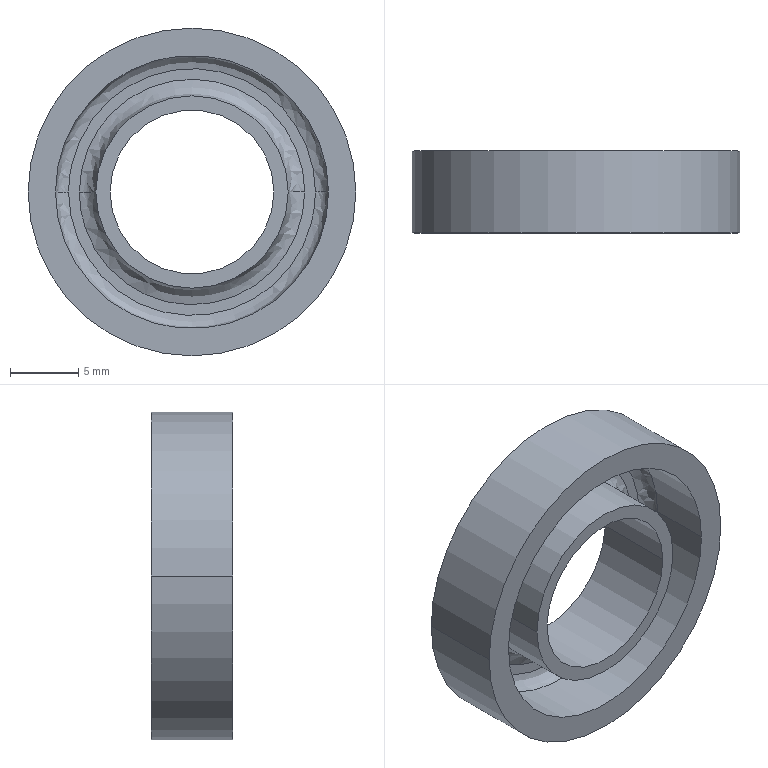Part | SolidWorks | features BaseBody 1 | 1 solid | 16 faces | box 24 x 6 x 24 mm | volume 1192 mm3 | cylinder 8 | spline 4 | plane 4 | commonest cylinder face diameters 12 x2 14.088 x2 20 x2 24 x2
STEP:
#1=CARTESIAN_POINT('',(-9.038,-85.,0.));
#2=VERTEX_POINT('',#1);
#3=CARTESIAN_POINT('',(9.038,-85.,0.));
#4=VERTEX_POINT('',#3);
#5=CARTESIAN_POINT('',(-9.038,-85.,0.));
#6=CARTESIAN_POINT('',(-9.038,-85.,-0.2762));
#7=CARTESIAN_POINT('',(-9.019,-85.,-0.6889));
#8=CARTESIAN_POINT('',(-8.964,-85.,-1.168));
#9=CARTESIAN_POINT('',(-8.928,-85.,-1.406));
#10=CARTESIAN_POINT('',(-8.911,-85.,-1.508));
#11=CARTESIAN_POINT('',(-8.899,-85.,-1.577));
#12=CARTESIAN_POINT('',(-8.893,-85.,-1.609));
#13=CARTESIAN_POINT('',(-8.834,-85.,-1.933));
#14=CARTESIAN_POINT('',(-8.733,-85.,-2.359));
#15=CARTESIAN_POINT('',(-8.58,-85.,-2.846));
#16=CARTESIAN_POINT('',(-8.495,-85.,-3.087));
#17=CARTESIAN_POINT('',(-8.456,-85.,-3.19));
#18=CARTESIAN_POINT('',(-8.43,-85.,-3.259));
#19=CARTESIAN_POINT('',(-8.417,-85.,-3.291));
#20=CARTESIAN_POINT('',(-8.291,-85.,-3.611));
#21=CARTESIAN_POINT('',(-8.102,-85.,-4.026));
#22=CARTESIAN_POINT('',(-7.845,-85.,-4.492));
#23=CARTESIAN_POINT('',(-7.727,-85.,-4.688));
#24=CARTESIAN_POINT('',(-7.647,-85.,-4.817));
#25=CARTESIAN_POINT('',(-7.607,-85.,-4.88));
#26=CARTESIAN_POINT('',(-7.223,-85.,-5.467));
#27=CARTESIAN_POINT('',(-6.832,-85.,-5.95));
#28=CARTESIAN_POINT('',(-6.17,-85.,-6.611));
#29=CARTESIAN_POINT('',(-5.824,-85.,-6.923));
#30=CARTESIAN_POINT('',(-5.394,-85.,-7.255));
#31=CARTESIAN_POINT('',(-5.204,-85.,-7.39));
#32=CARTESIAN_POINT('',(-5.076,-85.,-7.478));
#33=CARTESIAN_POINT('',(-5.009,-85.,-7.523));
#34=CARTESIAN_POINT('',(-4.69,-85.,-7.732));
#35=CARTESIAN_POINT('',(-4.296,-85.,-7.962));
#36=CARTESIAN_POINT('',(-3.818,-85.,-8.194));
#37=CARTESIAN_POINT('',(-3.574,-85.,-8.302));
#38=CARTESIAN_POINT('',(-3.468,-85.,-8.346));
#39=CARTESIAN_POINT('',(-3.398,-85.,-8.375));
#40=CARTESIAN_POINT('',(-3.361,-85.,-8.39));
#41=CARTESIAN_POINT('',(-3.054,-85.,-8.511));
#42=CARTESIAN_POINT('',(-2.64,-85.,-8.652));
#43=CARTESIAN_POINT('',(-2.146,-85.,-8.781));
#44=CARTESIAN_POINT('',(-1.896,-85.,-8.837));
#45=CARTESIAN_POINT('',(-1.788,-85.,-8.859));
#46=CARTESIAN_POINT('',(-1.717,-85.,-8.873));
#47=CARTESIAN_POINT('',(-1.678,-85.,-8.881));
#48=CARTESIAN_POINT('',(-1.101,-85.,-8.987));
#49=CARTESIAN_POINT('',(-0.5524,-85.,-9.038));
#50=CARTESIAN_POINT('',(0.2762,-85.,-9.038));
#51=CARTESIAN_POINT('',(0.6889,-85.,-9.019));
#52=CARTESIAN_POINT('',(1.168,-85.,-8.964));
#53=CARTESIAN_POINT('',(1.406,-85.,-8.928));
#54=CARTESIAN_POINT('',(1.508,-85.,-8.911));
#55=CARTESIAN_POINT('',(1.577,-85.,-8.899));
#56=CARTESIAN_POINT('',(1.609,-85.,-8.893));
#57=CARTESIAN_POINT('',(1.933,-85.,-8.834));
#58=CARTESIAN_POINT('',(2.359,-85.,-8.733));
#59=CARTESIAN_POINT('',(2.846,-85.,-8.58));
#60=CARTESIAN_POINT('',(3.087,-85.,-8.495));
#61=CARTESIAN_POINT('',(3.19,-85.,-8.456));
#62=CARTESIAN_POINT('',(3.259,-85.,-8.43));
#63=CARTESIAN_POINT('',(3.291,-85.,-8.417));
#64=CARTESIAN_POINT('',(3.611,-85.,-8.291));
#65=CARTESIAN_POINT('',(4.026,-85.,-8.102));
#66=CARTESIAN_POINT('',(4.492,-85.,-7.845));
#67=CARTESIAN_POINT('',(4.688,-85.,-7.727));
#68=CARTESIAN_POINT('',(4.817,-85.,-7.647));
#69=CARTESIAN_POINT('',(4.88,-85.,-7.607));
#70=CARTESIAN_POINT('',(5.467,-85.,-7.223));
#71=CARTESIAN_POINT('',(5.95,-85.,-6.832));
#72=CARTESIAN_POINT('',(6.611,-85.,-6.17));
#73=CARTESIAN_POINT('',(6.923,-85.,-5.824));
#74=CARTESIAN_POINT('',(7.255,-85.,-5.394));
#75=CARTESIAN_POINT('',(7.39,-85.,-5.204));
#76=CARTESIAN_POINT('',(7.478,-85.,-5.076));
#77=CARTESIAN_POINT('',(7.523,-85.,-5.009));
#78=CARTESIAN_POINT('',(7.732,-85.,-4.69));
#79=CARTESIAN_POINT('',(7.962,-85.,-4.296));
#80=CARTESIAN_POINT('',(8.194,-85.,-3.818));
#81=CARTESIAN_POINT('',(8.302,-85.,-3.574));
#82=CARTESIAN_POINT('',(8.346,-85.,-3.468));
#83=CARTESIAN_POINT('',(8.375,-85.,-3.398));
#84=CARTESIAN_POINT('',(8.39,-85.,-3.361));
#85=CARTESIAN_POINT('',(8.511,-85.,-3.054));
#86=CARTESIAN_POINT('',(8.652,-85.,-2.64));
#87=CARTESIAN_POINT('',(8.781,-85.,-2.146));
#88=CARTESIAN_POINT('',(8.837,-85.,-1.896));
#89=CARTESIAN_POINT('',(8.859,-85.,-1.788));
#90=CARTESIAN_POINT('',(8.873,-85.,-1.717));
#91=CARTESIAN_POINT('',(8.881,-85.,-1.678));
#92=CARTESIAN_POINT('',(8.987,-85.,-1.101));
#93=CARTESIAN_POINT('',(9.038,-85.,-0.5524));
#94=CARTESIAN_POINT('',(9.038,-85.,0.));
#95=B_SPLINE_CURVE_WITH_KNOTS('',3,(#5,#6,#7,#8,#9,#10,#11,#12,#13,#14,#15,#16,#17,#18,#19,#20,#21,#22,#23,#24,#25,#26,#27,#28,#29,#30,#31,#32,#33,#34,#35,#36,#37,#38,#39,#40,#41,#42,#43,#44,#45,#46,#47,#48,#49,#50,#51,#52,#53,#54,#55,#56,#57,#58,#59,#60,#61,#62,#63,#64,#65,#66,#67,#68,#69,#70,#71,#72,#73,#74,#75,#76,#77,#78,#79,#80,#81,#82,#83,#84,#85,#86,#87,#88,#89,#90,#91,#92,#93,#94),.UNSPECIFIED.,.F.,.F.,(4,1,1,1,2,2,1,1,1,2,2,1,1,2,2,2,1,1,2,2,1,1,1,2,2,1,1,1,2,2,2,1,1,1,2,2,1,1,1,2,2,1,1,2,2,2,1,1,2,2,1,1,1,2,2,1,1,1,2,2,4),(0.25,0.2656,0.2734,0.2773,0.2793,0.2813,0.2969,0.3047,0.3086,0.3105,0.3125,0.3281,0.3359,0.3398,0.3438,0.375,0.3906,0.3984,0.4023,0.4063,0.4219,0.4297,0.4336,0.4355,0.4375,0.4531,0.4609,0.4648,0.4668,0.4688,0.5,0.5156,0.5234,0.5273,0.5293,0.5313,0.5469,0.5547,0.5586,0.5605,0.5625,0.5781,0.5859,0.5898,0.5938,0.625,0.6406,0.6484,0.6523,0.6563,0.6719,0.6797,0.6836,0.6855,0.6875,0.7031,0.7109,0.7148,0.7168,0.7188,0.75),.UNSPECIFIED.);
#96=EDGE_CURVE('',#2,#4,#95,.T.);
#97=ORIENTED_EDGE('',*,*,#96,.F.);
#98=CARTESIAN_POINT('',(-10.,-85.962,0.));
#99=VERTEX_POINT('',#98);
#100=CARTESIAN_POINT('',(-9.038,-85.962,0.));
#101=DIRECTION('',(0.,0.,1.));
#102=DIRECTION('',(-1.,0.,0.));
#103=AXIS2_PLACEMENT_3D('',#100,#101,#102);
#104=CIRCLE('',#103,0.9623);
#105=EDGE_CURVE('',#2,#99,#104,.T.);
#106=ORIENTED_EDGE('',*,*,#105,.T.);
#107=CARTESIAN_POINT('',(10.,-85.962,0.));
#108=VERTEX_POINT('',#107);
#109=CARTESIAN_POINT('',(0.,-85.962,0.));
#110=DIRECTION('',(0.,-1.,0.));
#111=DIRECTION('',(-1.,0.,0.));
#112=AXIS2_PLACEMENT_3D('',#109,#110,#111);
#113=CIRCLE('',#112,10.);
#114=EDGE_CURVE('',#99,#108,#113,.T.);
#115=ORIENTED_EDGE('',*,*,#114,.T.);
#116=CARTESIAN_POINT('',(9.038,-85.962,0.));
#117=DIRECTION('',(0.,0.,-1.));
#118=DIRECTION('',(1.,0.,0.));
#119=AXIS2_PLACEMENT_3D('',#116,#117,#118);
#120=CIRCLE('',#119,0.9623);
#121=EDGE_CURVE('',#4,#108,#120,.T.);
#122=ORIENTED_EDGE('',*,*,#121,.F.);
#123=EDGE_LOOP('',(#97,#106,#115,#122));
#124=FACE_OUTER_BOUND('',#123,.T.);
#125=CARTESIAN_POINT('',(9.038,-85.,0.));
#126=CARTESIAN_POINT('',(9.038,-85.,-18.075));
#127=CARTESIAN_POINT('',(-9.038,-85.,-18.075));
#128=CARTESIAN_POINT('',(-9.038,-85.,0.));
#129=CARTESIAN_POINT('',(9.601,-85.,0.));
#130=CARTESIAN_POINT('',(9.601,-85.,-19.203));
#131=CARTESIAN_POINT('',(-9.601,-85.,-19.203));
#132=CARTESIAN_POINT('',(-9.601,-85.,0.));
#133=CARTESIAN_POINT('',(10.,-85.399,0.));
#134=CARTESIAN_POINT('',(10.,-85.399,-20.));
#135=CARTESIAN_POINT('',(-10.,-85.399,-20.));
#136=CARTESIAN_POINT('',(-10.,-85.399,0.));
#137=CARTESIAN_POINT('',(10.,-85.962,0.));
#138=CARTESIAN_POINT('',(10.,-85.962,-20.));
#139=CARTESIAN_POINT('',(-10.,-85.962,-20.));
#140=CARTESIAN_POINT('',(-10.,-85.962,0.));
#141=(BOUNDED_SURFACE()B_SPLINE_SURFACE(3,3,((#125,#126,#127,#128),(#129,#130,#131,#132),(#133,#134,#135,#136),(#137,#138,#139,#140)),.UNSPECIFIED.,.F.,.F.,.T.)B_SPLINE_SURFACE_WITH_KNOTS((4,4),(4,4),(0.,1.),(0.,1.),.UNSPECIFIED.)GEOMETRIC_REPRESENTATION_ITEM()RATIONAL_B_SPLINE_SURFACE(((1.,0.3333,0.3333,1.),(0.8047,0.2682,0.2682,0.8047),(0.8047,0.2682,0.2682,0.8047),(1.,0.3333,0.3333,1.)))REPRESENTATION_ITEM('')SURFACE());
#142=ADVANCED_FACE('',(#124),#141,.F.);
#143=CARTESIAN_POINT('',(-7.044,-86.21,0.));
#144=VERTEX_POINT('',#143);
#145=CARTESIAN_POINT('',(7.044,-86.21,0.));
#146=VERTEX_POINT('',#145);
#147=CARTESIAN_POINT('',(0.,-86.21,0.));
#148=DIRECTION('',(0.,-1.,0.));
#149=DIRECTION('',(-1.,0.,0.));
#150=AXIS2_PLACEMENT_3D('',#147,#148,#149);
#151=CIRCLE('',#150,7.044);
#152=EDGE_CURVE('',#144,#146,#151,.T.);
#153=ORIENTED_EDGE('',*,*,#152,.F.);
#154=CARTESIAN_POINT('',(-8.255,-85.,0.));
#155=VERTEX_POINT('',#154);
#156=CARTESIAN_POINT('',(-8.255,-86.21,0.));
#157=DIRECTION('',(0.,0.,1.));
#158=DIRECTION('',(-1.,0.,0.));
#159=AXIS2_PLACEMENT_3D('',#156,#157,#158);
#160=CIRCLE('',#159,1.21);
#161=EDGE_CURVE('',#144,#155,#160,.T.);
#162=ORIENTED_EDGE('',*,*,#161,.T.);
#163=CARTESIAN_POINT('',(8.255,-85.,0.));
#164=VERTEX_POINT('',#163);
#165=CARTESIAN_POINT('',(8.255,-85.,0.));
#166=CARTESIAN_POINT('',(8.255,-85.,-0.2523));
#167=CARTESIAN_POINT('',(8.237,-85.,-0.6292));
#168=CARTESIAN_POINT('',(8.187,-85.,-1.066));
#169=CARTESIAN_POINT('',(8.154,-85.,-1.284));
#170=CARTESIAN_POINT('',(8.139,-85.,-1.378));
#171=CARTESIAN_POINT('',(8.128,-85.,-1.44));
#172=CARTESIAN_POINT('',(8.123,-85.,-1.469));
#173=CARTESIAN_POINT('',(8.068,-85.,-1.765));
#174=CARTESIAN_POINT('',(7.976,-85.,-2.154));
#175=CARTESIAN_POINT('',(7.837,-85.,-2.599));
#176=CARTESIAN_POINT('',(7.758,-85.,-2.82));
#177=CARTESIAN_POINT('',(7.723,-85.,-2.914));
#178=CARTESIAN_POINT('',(7.699,-85.,-2.976));
#179=CARTESIAN_POINT('',(7.688,-85.,-3.006));
#180=CARTESIAN_POINT('',(7.572,-85.,-3.298));
#181=CARTESIAN_POINT('',(7.4,-85.,-3.677));
#182=CARTESIAN_POINT('',(7.165,-85.,-4.102));
#183=CARTESIAN_POINT('',(7.058,-85.,-4.281));
#184=CARTESIAN_POINT('',(6.985,-85.,-4.4));
#185=CARTESIAN_POINT('',(6.948,-85.,-4.457));
#186=CARTESIAN_POINT('',(6.597,-85.,-4.994));
#187=CARTESIAN_POINT('',(6.239,-85.,-5.434));
#188=CARTESIAN_POINT('',(5.635,-85.,-6.038));
#189=CARTESIAN_POINT('',(5.32,-85.,-6.323));
#190=CARTESIAN_POINT('',(4.926,-85.,-6.626));
#191=CARTESIAN_POINT('',(4.753,-85.,-6.749));
#192=CARTESIAN_POINT('',(4.636,-85.,-6.83));
#193=CARTESIAN_POINT('',(4.575,-85.,-6.871));
#194=CARTESIAN_POINT('',(4.284,-85.,-7.062));
#195=CARTESIAN_POINT('',(3.924,-85.,-7.272));
#196=CARTESIAN_POINT('',(3.487,-85.,-7.484));
#197=CARTESIAN_POINT('',(3.264,-85.,-7.582));
#198=CARTESIAN_POINT('',(3.168,-85.,-7.623));
#199=CARTESIAN_POINT('',(3.103,-85.,-7.649));
#200=CARTESIAN_POINT('',(3.07,-85.,-7.663));
#201=CARTESIAN_POINT('',(2.79,-85.,-7.773));
#202=CARTESIAN_POINT('',(2.411,-85.,-7.903));
#203=CARTESIAN_POINT('',(1.96,-85.,-8.02));
#204=CARTESIAN_POINT('',(1.732,-85.,-8.071));
#205=CARTESIAN_POINT('',(1.633,-85.,-8.091));
#206=CARTESIAN_POINT('',(1.568,-85.,-8.104));
#207=CARTESIAN_POINT('',(1.533,-85.,-8.111));
#208=CARTESIAN_POINT('',(1.006,-85.,-8.209));
#209=CARTESIAN_POINT('',(0.5045,-85.,-8.254));
#210=CARTESIAN_POINT('',(-0.2523,-85.,-8.255));
#211=CARTESIAN_POINT('',(-0.6292,-85.,-8.237));
#212=CARTESIAN_POINT('',(-1.066,-85.,-8.187));
#213=CARTESIAN_POINT('',(-1.284,-85.,-8.154));
#214=CARTESIAN_POINT('',(-1.378,-85.,-8.139));
#215=CARTESIAN_POINT('',(-1.44,-85.,-8.128));
#216=CARTESIAN_POINT('',(-1.469,-85.,-8.123));
#217=CARTESIAN_POINT('',(-1.765,-85.,-8.068));
#218=CARTESIAN_POINT('',(-2.154,-85.,-7.976));
#219=CARTESIAN_POINT('',(-2.599,-85.,-7.837));
#220=CARTESIAN_POINT('',(-2.82,-85.,-7.758));
#221=CARTESIAN_POINT('',(-2.914,-85.,-7.723));
#222=CARTESIAN_POINT('',(-2.976,-85.,-7.699));
#223=CARTESIAN_POINT('',(-3.006,-85.,-7.688));
#224=CARTESIAN_POINT('',(-3.298,-85.,-7.572));
#225=CARTESIAN_POINT('',(-3.677,-85.,-7.4));
#226=CARTESIAN_POINT('',(-4.102,-85.,-7.165));
#227=CARTESIAN_POINT('',(-4.281,-85.,-7.058));
#228=CARTESIAN_POINT('',(-4.4,-85.,-6.985));
#229=CARTESIAN_POINT('',(-4.457,-85.,-6.948));
#230=CARTESIAN_POINT('',(-4.994,-85.,-6.597));
#231=CARTESIAN_POINT('',(-5.434,-85.,-6.239));
#232=CARTESIAN_POINT('',(-6.038,-85.,-5.635));
#233=CARTESIAN_POINT('',(-6.323,-85.,-5.32));
#234=CARTESIAN_POINT('',(-6.626,-85.,-4.926));
#235=CARTESIAN_POINT('',(-6.749,-85.,-4.753));
#236=CARTESIAN_POINT('',(-6.83,-85.,-4.636));
#237=CARTESIAN_POINT('',(-6.871,-85.,-4.575));
#238=CARTESIAN_POINT('',(-7.062,-85.,-4.284));
#239=CARTESIAN_POINT('',(-7.272,-85.,-3.924));
#240=CARTESIAN_POINT('',(-7.484,-85.,-3.487));
#241=CARTESIAN_POINT('',(-7.582,-85.,-3.264));
#242=CARTESIAN_POINT('',(-7.623,-85.,-3.168));
#243=CARTESIAN_POINT('',(-7.649,-85.,-3.103));
#244=CARTESIAN_POINT('',(-7.663,-85.,-3.07));
#245=CARTESIAN_POINT('',(-7.773,-85.,-2.79));
#246=CARTESIAN_POINT('',(-7.903,-85.,-2.411));
#247=CARTESIAN_POINT('',(-8.02,-85.,-1.96));
#248=CARTESIAN_POINT('',(-8.071,-85.,-1.732));
#249=CARTESIAN_POINT('',(-8.091,-85.,-1.633));
#250=CARTESIAN_POINT('',(-8.104,-85.,-1.568));
#251=CARTESIAN_POINT('',(-8.111,-85.,-1.533));
#252=CARTESIAN_POINT('',(-8.209,-85.,-1.006));
#253=CARTESIAN_POINT('',(-8.254,-85.,-0.5045));
#254=CARTESIAN_POINT('',(-8.255,-85.,0.));
#255=B_SPLINE_CURVE_WITH_KNOTS('',3,(#165,#166,#167,#168,#169,#170,#171,#172,#173,#174,#175,#176,#177,#178,#179,#180,#181,#182,#183,#184,#185,#186,#187,#188,#189,#190,#191,#192,#193,#194,#195,#196,#197,#198,#199,#200,#201,#202,#203,#204,#205,#206,#207,#208,#209,#210,#211,#212,#213,#214,#215,#216,#217,#218,#219,#220,#221,#222,#223,#224,#225,#226,#227,#228,#229,#230,#231,#232,#233,#234,#235,#236,#237,#238,#239,#240,#241,#242,#243,#244,#245,#246,#247,#248,#249,#250,#251,#252,#253,#254),.UNSPECIFIED.,.F.,.F.,(4,1,1,1,2,2,1,1,1,2,2,1,1,2,2,2,1,1,2,2,1,1,1,2,2,1,1,1,2,2,2,1,1,1,2,2,1,1,1,2,2,1,1,2,2,2,1,1,2,2,1,1,1,2,2,1,1,1,2,2,4),(0.25,0.2656,0.2734,0.2773,0.2793,0.2812,0.2969,0.3047,0.3086,0.3105,0.3125,0.3281,0.3359,0.3398,0.3437,0.375,0.3906,0.3984,0.4023,0.4062,0.4219,0.4297,0.4336,0.4355,0.4375,0.4531,0.4609,0.4648,0.4668,0.4687,0.5,0.5156,0.5234,0.5273,0.5293,0.5313,0.5469,0.5547,0.5586,0.5605,0.5625,0.5781,0.5859,0.5898,0.5938,0.625,0.6406,0.6484,0.6523,0.6563,0.6719,0.6797,0.6836,0.6855,0.6875,0.7031,0.7109,0.7148,0.7168,0.7188,0.75),.UNSPECIFIED.);
#256=EDGE_CURVE('',#164,#155,#255,.T.);
#257=ORIENTED_EDGE('',*,*,#256,.F.);
#258=CARTESIAN_POINT('',(8.255,-86.21,0.));
#259=DIRECTION('',(0.,0.,-1.));
#260=DIRECTION('',(1.,0.,0.));
#261=AXIS2_PLACEMENT_3D('',#258,#259,#260);
#262=CIRCLE('',#261,1.21);
#263=EDGE_CURVE('',#146,#164,#262,.T.);
#264=ORIENTED_EDGE('',*,*,#263,.F.);
#265=EDGE_LOOP('',(#153,#162,#257,#264));
#266=FACE_OUTER_BOUND('',#265,.T.);
#267=CARTESIAN_POINT('',(7.044,-86.21,0.));
#268=CARTESIAN_POINT('',(7.044,-86.21,-14.088));
#269=CARTESIAN_POINT('',(-7.044,-86.21,-14.088));
#270=CARTESIAN_POINT('',(-7.044,-86.21,0.));
#271=CARTESIAN_POINT('',(7.044,-85.501,0.));
#272=CARTESIAN_POINT('',(7.044,-85.501,-14.088));
#273=CARTESIAN_POINT('',(-7.044,-85.501,-14.088));
#274=CARTESIAN_POINT('',(-7.044,-85.501,0.));
#275=CARTESIAN_POINT('',(7.546,-85.,0.));
#276=CARTESIAN_POINT('',(7.546,-85.,-15.091));
#277=CARTESIAN_POINT('',(-7.546,-85.,-15.091));
#278=CARTESIAN_POINT('',(-7.546,-85.,0.));
#279=CARTESIAN_POINT('',(8.255,-85.,0.));
#280=CARTESIAN_POINT('',(8.255,-85.,-16.509));
#281=CARTESIAN_POINT('',(-8.255,-85.,-16.509));
#282=CARTESIAN_POINT('',(-8.255,-85.,0.));
#283=(BOUNDED_SURFACE()B_SPLINE_SURFACE(3,3,((#267,#268,#269,#270),(#271,#272,#273,#274),(#275,#276,#277,#278),(#279,#280,#281,#282)),.UNSPECIFIED.,.F.,.F.,.F.)B_SPLINE_SURFACE_WITH_KNOTS((4,4),(4,4),(0.,1.),(0.,1.),.UNSPECIFIED.)GEOMETRIC_REPRESENTATION_ITEM()RATIONAL_B_SPLINE_SURFACE(((1.,0.3333,0.3333,1.),(0.8047,0.2682,0.2682,0.8047),(0.8047,0.2682,0.2682,0.8047),(1.,0.3333,0.3333,1.)))REPRESENTATION_ITEM('')SURFACE());
#284=ADVANCED_FACE('',(#266),#283,.F.);
#285=CARTESIAN_POINT('',(-12.,-90.5,0.));
#286=VERTEX_POINT('',#285);
#287=CARTESIAN_POINT('',(12.,-90.5,0.));
#288=VERTEX_POINT('',#287);
#289=CARTESIAN_POINT('',(0.,-90.5,0.));
#290=DIRECTION('',(0.,1.,0.));
#291=DIRECTION('',(-1.,0.,0.));
#292=AXIS2_PLACEMENT_3D('',#289,#290,#291);
#293=CIRCLE('',#292,12.);
#294=EDGE_CURVE('',#286,#288,#293,.T.);
#295=ORIENTED_EDGE('',*,*,#294,.T.);
#296=CARTESIAN_POINT('',(12.,-84.5,0.));
#297=VERTEX_POINT('',#296);
#298=CARTESIAN_POINT('',(12.,-83.5,0.));
#299=DIRECTION('',(0.,1.,0.));
#300=VECTOR('',#299,1000.);
#301=LINE('',#298,#300);
#302=EDGE_CURVE('',#288,#297,#301,.T.);
#303=ORIENTED_EDGE('',*,*,#302,.T.);
#304=CARTESIAN_POINT('',(-12.,-84.5,0.));
#305=VERTEX_POINT('',#304);
#306=CARTESIAN_POINT('',(0.,-84.5,0.));
#307=DIRECTION('',(0.,-1.,0.));
#308=DIRECTION('',(-1.,0.,0.));
#309=AXIS2_PLACEMENT_3D('',#306,#307,#308);
#310=CIRCLE('',#309,12.);
#311=EDGE_CURVE('',#297,#305,#310,.T.);
#312=ORIENTED_EDGE('',*,*,#311,.T.);
#313=CARTESIAN_POINT('',(-12.,-83.5,0.));
#314=DIRECTION('',(0.,1.,0.));
#315=VECTOR('',#314,1000.);
#316=LINE('',#313,#315);
#317=EDGE_CURVE('',#286,#305,#316,.T.);
#318=ORIENTED_EDGE('',*,*,#317,.F.);
#319=EDGE_LOOP('',(#295,#303,#312,#318));
#320=FACE_OUTER_BOUND('',#319,.T.);
#321=CARTESIAN_POINT('',(0.,-83.5,0.));
#322=DIRECTION('',(0.,1.,0.));
#323=DIRECTION('',(-1.,0.,0.));
#324=AXIS2_PLACEMENT_3D('',#321,#322,#323);
#325=CYLINDRICAL_SURFACE('',#324,12.);
#326=ADVANCED_FACE('',(#320),#325,.T.);
#327=CARTESIAN_POINT('',(6.,-90.5,0.));
#328=VERTEX_POINT('',#327);
#329=CARTESIAN_POINT('',(-6.,-90.5,0.));
#330=VERTEX_POINT('',#329);
#331=CARTESIAN_POINT('',(0.,-90.5,0.));
#332=DIRECTION('',(0.,1.,0.));
#333=DIRECTION('',(-1.,0.,0.));
#334=AXIS2_PLACEMENT_3D('',#331,#332,#333);
#335=CIRCLE('',#334,6.);
#336=EDGE_CURVE('',#328,#330,#335,.T.);
#337=ORIENTED_EDGE('',*,*,#336,.F.);
#338=CARTESIAN_POINT('',(6.,-84.5,0.));
#339=VERTEX_POINT('',#338);
#340=CARTESIAN_POINT('',(6.,-83.5,0.));
#341=DIRECTION('',(0.,1.,0.));
#342=VECTOR('',#341,1000.);
#343=LINE('',#340,#342);
#344=EDGE_CURVE('',#328,#339,#343,.T.);
#345=ORIENTED_EDGE('',*,*,#344,.T.);
#346=CARTESIAN_POINT('',(-6.,-84.5,0.));
#347=VERTEX_POINT('',#346);
#348=CARTESIAN_POINT('',(0.,-84.5,0.));
#349=DIRECTION('',(0.,-1.,0.));
#350=DIRECTION('',(-1.,0.,0.));
#351=AXIS2_PLACEMENT_3D('',#348,#349,#350);
#352=CIRCLE('',#351,6.);
#353=EDGE_CURVE('',#347,#339,#352,.T.);
#354=ORIENTED_EDGE('',*,*,#353,.F.);
#355=CARTESIAN_POINT('',(-6.,-83.5,0.));
#356=DIRECTION('',(0.,1.,0.));
#357=VECTOR('',#356,1000.);
#358=LINE('',#355,#357);
#359=EDGE_CURVE('',#330,#347,#358,.T.);
#360=ORIENTED_EDGE('',*,*,#359,.F.);
#361=EDGE_LOOP('',(#337,#345,#354,#360));
#362=FACE_OUTER_BOUND('',#361,.T.);
#363=CARTESIAN_POINT('',(0.,-83.5,0.));
#364=DIRECTION('',(0.,1.,0.));
#365=DIRECTION('',(-1.,0.,0.));
#366=AXIS2_PLACEMENT_3D('',#363,#364,#365);
#367=CYLINDRICAL_SURFACE('',#366,6.);
#368=ADVANCED_FACE('',(#362),#367,.F.);
#369=CARTESIAN_POINT('',(10.,-90.5,0.));
#370=VERTEX_POINT('',#369);
#371=CARTESIAN_POINT('',(-10.,-90.5,0.));
#372=VERTEX_POINT('',#371);
#373=CARTESIAN_POINT('',(0.,-90.5,0.));
#374=DIRECTION('',(0.,1.,0.));
#375=DIRECTION('',(-1.,0.,0.));
#376=AXIS2_PLACEMENT_3D('',#373,#374,#375);
#377=CIRCLE('',#376,10.);
#378=EDGE_CURVE('',#370,#372,#377,.T.);
#379=ORIENTED_EDGE('',*,*,#378,.F.);
#380=CARTESIAN_POINT('',(10.,-83.5,0.));
#381=DIRECTION('',(0.,1.,0.));
#382=VECTOR('',#381,1000.);
#383=LINE('',#380,#382);
#384=EDGE_CURVE('',#370,#108,#383,.T.);
#385=ORIENTED_EDGE('',*,*,#384,.T.);
#386=ORIENTED_EDGE('',*,*,#114,.F.);
#387=CARTESIAN_POINT('',(-10.,-83.5,0.));
#388=DIRECTION('',(0.,1.,0.));
#389=VECTOR('',#388,1000.);
#390=LINE('',#387,#389);
#391=EDGE_CURVE('',#372,#99,#390,.T.);
#392=ORIENTED_EDGE('',*,*,#391,.F.);
#393=EDGE_LOOP('',(#379,#385,#386,#392));
#394=FACE_OUTER_BOUND('',#393,.T.);
#395=CARTESIAN_POINT('',(0.,-83.5,0.));
#396=DIRECTION('',(0.,1.,0.));
#397=DIRECTION('',(-1.,0.,0.));
#398=AXIS2_PLACEMENT_3D('',#395,#396,#397);
#399=CYLINDRICAL_SURFACE('',#398,10.);
#400=ADVANCED_FACE('',(#394),#399,.F.);
#401=CARTESIAN_POINT('',(7.044,-90.5,0.));
#402=VERTEX_POINT('',#401);
#403=CARTESIAN_POINT('',(-7.044,-90.5,0.));
#404=VERTEX_POINT('',#403);
#405=CARTESIAN_POINT('',(0.,-90.5,0.));
#406=DIRECTION('',(0.,-1.,0.));
#407=DIRECTION('',(-1.,0.,0.));
#408=AXIS2_PLACEMENT_3D('',#405,#406,#407);
#409=CIRCLE('',#408,7.044);
#410=EDGE_CURVE('',#402,#404,#409,.T.);
#411=ORIENTED_EDGE('',*,*,#410,.F.);
#412=CARTESIAN_POINT('',(7.044,-83.5,0.));
#413=DIRECTION('',(0.,1.,0.));
#414=VECTOR('',#413,1000.);
#415=LINE('',#412,#414);
#416=EDGE_CURVE('',#402,#146,#415,.T.);
#417=ORIENTED_EDGE('',*,*,#416,.T.);
#418=CARTESIAN_POINT('',(0.,-86.21,0.));
#419=DIRECTION('',(0.,-1.,0.));
#420=DIRECTION('',(-1.,0.,0.));
#421=AXIS2_PLACEMENT_3D('',#418,#419,#420);
#422=CIRCLE('',#421,7.044);
#423=EDGE_CURVE('',#146,#144,#422,.T.);
#424=ORIENTED_EDGE('',*,*,#423,.T.);
#425=CARTESIAN_POINT('',(-7.044,-83.5,0.));
#426=DIRECTION('',(0.,1.,0.));
#427=VECTOR('',#426,1000.);
#428=LINE('',#425,#427);
#429=EDGE_CURVE('',#404,#144,#428,.T.);
#430=ORIENTED_EDGE('',*,*,#429,.F.);
#431=EDGE_LOOP('',(#411,#417,#424,#430));
#432=FACE_OUTER_BOUND('',#431,.T.);
#433=CARTESIAN_POINT('',(0.,-83.5,0.));
#434=DIRECTION('',(0.,1.,0.));
#435=DIRECTION('',(-1.,0.,0.));
#436=AXIS2_PLACEMENT_3D('',#433,#434,#435);
#437=CYLINDRICAL_SURFACE('',#436,7.044);
#438=ADVANCED_FACE('',(#432),#437,.T.);
#439=ORIENTED_EDGE('',*,*,#302,.F.);
#440=CARTESIAN_POINT('',(0.,-90.5,0.));
#441=DIRECTION('',(0.,1.,0.));
#442=DIRECTION('',(-1.,0.,0.));
#443=AXIS2_PLACEMENT_3D('',#440,#441,#442);
#444=CIRCLE('',#443,12.);
#445=EDGE_CURVE('',#288,#286,#444,.T.);
#446=ORIENTED_EDGE('',*,*,#445,.T.);
#447=ORIENTED_EDGE('',*,*,#317,.T.);
#448=CARTESIAN_POINT('',(0.,-84.5,0.));
#449=DIRECTION('',(0.,-1.,0.));
#450=DIRECTION('',(-1.,0.,0.));
#451=AXIS2_PLACEMENT_3D('',#448,#449,#450);
#452=CIRCLE('',#451,12.);
#453=EDGE_CURVE('',#305,#297,#452,.T.);
#454=ORIENTED_EDGE('',*,*,#453,.T.);
#455=EDGE_LOOP('',(#439,#446,#447,#454));
#456=FACE_OUTER_BOUND('',#455,.T.);
#457=CARTESIAN_POINT('',(0.,-83.5,0.));
#458=DIRECTION('',(0.,1.,0.));
#459=DIRECTION('',(-1.,0.,0.));
#460=AXIS2_PLACEMENT_3D('',#457,#458,#459);
#461=CYLINDRICAL_SURFACE('',#460,12.);
#462=ADVANCED_FACE('',(#456),#461,.T.);
#463=ORIENTED_EDGE('',*,*,#353,.T.);
#464=CARTESIAN_POINT('',(0.,-84.5,0.));
#465=DIRECTION('',(0.,-1.,0.));
#466=DIRECTION('',(-1.,0.,0.));
#467=AXIS2_PLACEMENT_3D('',#464,#465,#466);
#468=CIRCLE('',#467,6.);
#469=EDGE_CURVE('',#339,#347,#468,.T.);
#470=ORIENTED_EDGE('',*,*,#469,.T.);
#471=EDGE_LOOP('',(#463,#470));
#472=FACE_BOUND('',#471,.T.);
#473=ORIENTED_EDGE('',*,*,#453,.F.);
#474=ORIENTED_EDGE('',*,*,#311,.F.);
#475=EDGE_LOOP('',(#473,#474));
#476=FACE_OUTER_BOUND('',#475,.T.);
#477=CARTESIAN_POINT('',(0.,-84.5,6.));
#478=DIRECTION('',(0.,1.,0.));
#479=DIRECTION('',(-1.,0.,0.));
#480=AXIS2_PLACEMENT_3D('',#477,#478,#479);
#481=PLANE('',#480);
#482=ADVANCED_FACE('',(#472,#476),#481,.T.);
#483=ORIENTED_EDGE('',*,*,#294,.F.);
#484=ORIENTED_EDGE('',*,*,#445,.F.);
#485=EDGE_LOOP('',(#483,#484));
#486=FACE_OUTER_BOUND('',#485,.T.);
#487=CARTESIAN_POINT('',(0.,-90.5,0.));
#488=DIRECTION('',(0.,1.,0.));
#489=DIRECTION('',(-1.,0.,0.));
#490=AXIS2_PLACEMENT_3D('',#487,#488,#489);
#491=CIRCLE('',#490,10.);
#492=EDGE_CURVE('',#372,#370,#491,.T.);
#493=ORIENTED_EDGE('',*,*,#492,.T.);
#494=ORIENTED_EDGE('',*,*,#378,.T.);
#495=EDGE_LOOP('',(#493,#494));
#496=FACE_BOUND('',#495,.T.);
#497=CARTESIAN_POINT('',(0.,-90.5,12.));
#498=DIRECTION('',(0.,-1.,0.));
#499=DIRECTION('',(1.,0.,0.));
#500=AXIS2_PLACEMENT_3D('',#497,#498,#499);
#501=PLANE('',#500);
#502=ADVANCED_FACE('',(#486,#496),#501,.T.);
#503=ORIENTED_EDGE('',*,*,#344,.F.);
#504=CARTESIAN_POINT('',(0.,-90.5,0.));
#505=DIRECTION('',(0.,1.,0.));
#506=DIRECTION('',(-1.,0.,0.));
#507=AXIS2_PLACEMENT_3D('',#504,#505,#506);
#508=CIRCLE('',#507,6.);
#509=EDGE_CURVE('',#330,#328,#508,.T.);
#510=ORIENTED_EDGE('',*,*,#509,.F.);
#511=ORIENTED_EDGE('',*,*,#359,.T.);
#512=ORIENTED_EDGE('',*,*,#469,.F.);
#513=EDGE_LOOP('',(#503,#510,#511,#512));
#514=FACE_OUTER_BOUND('',#513,.T.);
#515=CARTESIAN_POINT('',(0.,-83.5,0.));
#516=DIRECTION('',(0.,1.,0.));
#517=DIRECTION('',(-1.,0.,0.));
#518=AXIS2_PLACEMENT_3D('',#515,#516,#517);
#519=CYLINDRICAL_SURFACE('',#518,6.);
#520=ADVANCED_FACE('',(#514),#519,.F.);
#521=ORIENTED_EDGE('',*,*,#384,.F.);
#522=ORIENTED_EDGE('',*,*,#492,.F.);
#523=ORIENTED_EDGE('',*,*,#391,.T.);
#524=CARTESIAN_POINT('',(0.,-85.962,0.));
#525=DIRECTION('',(0.,-1.,0.));
#526=DIRECTION('',(-1.,0.,0.));
#527=AXIS2_PLACEMENT_3D('',#524,#525,#526);
#528=CIRCLE('',#527,10.);
#529=EDGE_CURVE('',#108,#99,#528,.T.);
#530=ORIENTED_EDGE('',*,*,#529,.F.);
#531=EDGE_LOOP('',(#521,#522,#523,#530));
#532=FACE_OUTER_BOUND('',#531,.T.);
#533=CARTESIAN_POINT('',(0.,-83.5,0.));
#534=DIRECTION('',(0.,1.,0.));
#535=DIRECTION('',(-1.,0.,0.));
#536=AXIS2_PLACEMENT_3D('',#533,#534,#535);
#537=CYLINDRICAL_SURFACE('',#536,10.);
#538=ADVANCED_FACE('',(#532),#537,.F.);
#539=CARTESIAN_POINT('',(0.,-90.5,0.));
#540=DIRECTION('',(0.,-1.,0.));
#541=DIRECTION('',(-1.,0.,0.));
#542=AXIS2_PLACEMENT_3D('',#539,#540,#541);
#543=CIRCLE('',#542,7.044);
#544=EDGE_CURVE('',#404,#402,#543,.T.);
#545=ORIENTED_EDGE('',*,*,#544,.T.);
#546=ORIENTED_EDGE('',*,*,#410,.T.);
#547=EDGE_LOOP('',(#545,#546));
#548=FACE_OUTER_BOUND('',#547,.T.);
#549=ORIENTED_EDGE('',*,*,#509,.T.);
#550=ORIENTED_EDGE('',*,*,#336,.T.);
#551=EDGE_LOOP('',(#549,#550));
#552=FACE_BOUND('',#551,.T.);
#553=CARTESIAN_POINT('',(0.,-90.5,7.044));
#554=DIRECTION('',(0.,-1.,0.));
#555=DIRECTION('',(1.,0.,0.));
#556=AXIS2_PLACEMENT_3D('',#553,#554,#555);
#557=PLANE('',#556);
#558=ADVANCED_FACE('',(#548,#552),#557,.T.);
#559=ORIENTED_EDGE('',*,*,#105,.F.);
#560=CARTESIAN_POINT('',(9.038,-85.,0.));
#561=CARTESIAN_POINT('',(9.038,-85.,0.2762));
#562=CARTESIAN_POINT('',(9.019,-85.,0.6889));
#563=CARTESIAN_POINT('',(8.964,-85.,1.168));
#564=CARTESIAN_POINT('',(8.928,-85.,1.406));
#565=CARTESIAN_POINT('',(8.911,-85.,1.508));
#566=CARTESIAN_POINT('',(8.899,-85.,1.577));
#567=CARTESIAN_POINT('',(8.893,-85.,1.609));
#568=CARTESIAN_POINT('',(8.834,-85.,1.933));
#569=CARTESIAN_POINT('',(8.733,-85.,2.359));
#570=CARTESIAN_POINT('',(8.58,-85.,2.846));
#571=CARTESIAN_POINT('',(8.495,-85.,3.087));
#572=CARTESIAN_POINT('',(8.456,-85.,3.19));
#573=CARTESIAN_POINT('',(8.43,-85.,3.259));
#574=CARTESIAN_POINT('',(8.417,-85.,3.291));
#575=CARTESIAN_POINT('',(8.291,-85.,3.611));
#576=CARTESIAN_POINT('',(8.102,-85.,4.026));
#577=CARTESIAN_POINT('',(7.845,-85.,4.492));
#578=CARTESIAN_POINT('',(7.727,-85.,4.688));
#579=CARTESIAN_POINT('',(7.647,-85.,4.817));
#580=CARTESIAN_POINT('',(7.607,-85.,4.88));
#581=CARTESIAN_POINT('',(7.223,-85.,5.467));
#582=CARTESIAN_POINT('',(6.832,-85.,5.95));
#583=CARTESIAN_POINT('',(6.17,-85.,6.611));
#584=CARTESIAN_POINT('',(5.824,-85.,6.923));
#585=CARTESIAN_POINT('',(5.394,-85.,7.255));
#586=CARTESIAN_POINT('',(5.204,-85.,7.39));
#587=CARTESIAN_POINT('',(5.076,-85.,7.478));
#588=CARTESIAN_POINT('',(5.009,-85.,7.523));
#589=CARTESIAN_POINT('',(4.69,-85.,7.732));
#590=CARTESIAN_POINT('',(4.296,-85.,7.962));
#591=CARTESIAN_POINT('',(3.818,-85.,8.194));
#592=CARTESIAN_POINT('',(3.574,-85.,8.302));
#593=CARTESIAN_POINT('',(3.468,-85.,8.346));
#594=CARTESIAN_POINT('',(3.398,-85.,8.375));
#595=CARTESIAN_POINT('',(3.361,-85.,8.39));
#596=CARTESIAN_POINT('',(3.054,-85.,8.511));
#597=CARTESIAN_POINT('',(2.64,-85.,8.652));
#598=CARTESIAN_POINT('',(2.146,-85.,8.781));
#599=CARTESIAN_POINT('',(1.896,-85.,8.837));
#600=CARTESIAN_POINT('',(1.788,-85.,8.859));
#601=CARTESIAN_POINT('',(1.717,-85.,8.873));
#602=CARTESIAN_POINT('',(1.678,-85.,8.881));
#603=CARTESIAN_POINT('',(1.101,-85.,8.987));
#604=CARTESIAN_POINT('',(0.553,-85.,9.038));
#605=CARTESIAN_POINT('',(-0.2765,-85.,9.038));
#606=CARTESIAN_POINT('',(-0.5515,-85.,9.025));
#607=CARTESIAN_POINT('',(-0.9626,-85.,8.987));
#608=CARTESIAN_POINT('',(-1.168,-85.,8.964));
#609=CARTESIAN_POINT('',(-1.406,-85.,8.928));
#610=CARTESIAN_POINT('',(-1.509,-85.,8.911));
#611=CARTESIAN_POINT('',(-1.577,-85.,8.899));
#612=CARTESIAN_POINT('',(-1.609,-85.,8.893));
#613=CARTESIAN_POINT('',(-1.933,-85.,8.834));
#614=CARTESIAN_POINT('',(-2.359,-85.,8.733));
#615=CARTESIAN_POINT('',(-2.846,-85.,8.58));
#616=CARTESIAN_POINT('',(-3.087,-85.,8.495));
#617=CARTESIAN_POINT('',(-3.19,-85.,8.456));
#618=CARTESIAN_POINT('',(-3.259,-85.,8.43));
#619=CARTESIAN_POINT('',(-3.291,-85.,8.417));
#620=CARTESIAN_POINT('',(-3.611,-85.,8.291));
#621=CARTESIAN_POINT('',(-4.026,-85.,8.102));
#622=CARTESIAN_POINT('',(-4.492,-85.,7.845));
#623=CARTESIAN_POINT('',(-4.688,-85.,7.727));
#624=CARTESIAN_POINT('',(-4.817,-85.,7.647));
#625=CARTESIAN_POINT('',(-4.88,-85.,7.607));
#626=CARTESIAN_POINT('',(-5.467,-85.,7.223));
#627=CARTESIAN_POINT('',(-5.95,-85.,6.832));
#628=CARTESIAN_POINT('',(-6.611,-85.,6.17));
#629=CARTESIAN_POINT('',(-6.923,-85.,5.824));
#630=CARTESIAN_POINT('',(-7.255,-85.,5.394));
#631=CARTESIAN_POINT('',(-7.39,-85.,5.204));
#632=CARTESIAN_POINT('',(-7.478,-85.,5.076));
#633=CARTESIAN_POINT('',(-7.523,-85.,5.009));
#634=CARTESIAN_POINT('',(-7.732,-85.,4.69));
#635=CARTESIAN_POINT('',(-7.962,-85.,4.296));
#636=CARTESIAN_POINT('',(-8.194,-85.,3.818));
#637=CARTESIAN_POINT('',(-8.302,-85.,3.574));
#638=CARTESIAN_POINT('',(-8.346,-85.,3.468));
#639=CARTESIAN_POINT('',(-8.375,-85.,3.398));
#640=CARTESIAN_POINT('',(-8.39,-85.,3.361));
#641=CARTESIAN_POINT('',(-8.511,-85.,3.054));
#642=CARTESIAN_POINT('',(-8.652,-85.,2.64));
#643=CARTESIAN_POINT('',(-8.781,-85.,2.146));
#644=CARTESIAN_POINT('',(-8.837,-85.,1.896));
#645=CARTESIAN_POINT('',(-8.859,-85.,1.788));
#646=CARTESIAN_POINT('',(-8.873,-85.,1.717));
#647=CARTESIAN_POINT('',(-8.881,-85.,1.678));
#648=CARTESIAN_POINT('',(-8.987,-85.,1.101));
#649=CARTESIAN_POINT('',(-9.038,-85.,0.5524));
#650=CARTESIAN_POINT('',(-9.038,-85.,0.));
#651=B_SPLINE_CURVE_WITH_KNOTS('',3,(#560,#561,#562,#563,#564,#565,#566,#567,#568,#569,#570,#571,#572,#573,#574,#575,#576,#577,#578,#579,#580,#581,#582,#583,#584,#585,#586,#587,#588,#589,#590,#591,#592,#593,#594,#595,#596,#597,#598,#599,#600,#601,#602,#603,#604,#605,#606,#607,#608,#609,#610,#611,#612,#613,#614,#615,#616,#617,#618,#619,#620,#621,#622,#623,#624,#625,#626,#627,#628,#629,#630,#631,#632,#633,#634,#635,#636,#637,#638,#639,#640,#641,#642,#643,#644,#645,#646,#647,#648,#649,#650),.UNSPECIFIED.,.F.,.F.,(4,1,1,1,2,2,1,1,1,2,2,1,1,2,2,2,1,1,2,2,1,1,1,2,2,1,1,1,2,2,2,2,1,1,2,2,1,1,1,2,2,1,1,2,2,2,1,1,2,2,1,1,1,2,2,1,1,1,2,2,4),(0.75,0.7656,0.7734,0.7773,0.7793,0.7813,0.7969,0.8047,0.8086,0.8105,0.8125,0.8281,0.8359,0.8398,0.8438,0.875,0.8906,0.8984,0.9023,0.9063,0.9219,0.9297,0.9336,0.9355,0.9375,0.9531,0.9609,0.9648,0.9668,0.9688,1.,1.016,1.023,1.027,1.029,1.031,1.047,1.055,1.059,1.061,1.063,1.078,1.086,1.09,1.094,1.125,1.141,1.148,1.152,1.156,1.172,1.18,1.184,1.186,1.188,1.203,1.211,1.215,1.217,1.219,1.25),.UNSPECIFIED.);
#652=EDGE_CURVE('',#4,#2,#651,.T.);
#653=ORIENTED_EDGE('',*,*,#652,.F.);
#654=ORIENTED_EDGE('',*,*,#121,.T.);
#655=ORIENTED_EDGE('',*,*,#529,.T.);
#656=EDGE_LOOP('',(#559,#653,#654,#655));
#657=FACE_OUTER_BOUND('',#656,.T.);
#658=CARTESIAN_POINT('',(-9.038,-85.,0.));
#659=CARTESIAN_POINT('',(-9.038,-85.,18.075));
#660=CARTESIAN_POINT('',(9.038,-85.,18.075));
#661=CARTESIAN_POINT('',(9.038,-85.,0.));
#662=CARTESIAN_POINT('',(-9.601,-85.,0.));
#663=CARTESIAN_POINT('',(-9.601,-85.,19.203));
#664=CARTESIAN_POINT('',(9.601,-85.,19.203));
#665=CARTESIAN_POINT('',(9.601,-85.,0.));
#666=CARTESIAN_POINT('',(-10.,-85.399,0.));
#667=CARTESIAN_POINT('',(-10.,-85.399,20.));
#668=CARTESIAN_POINT('',(10.,-85.399,20.));
#669=CARTESIAN_POINT('',(10.,-85.399,0.));
#670=CARTESIAN_POINT('',(-10.,-85.962,0.));
#671=CARTESIAN_POINT('',(-10.,-85.962,20.));
#672=CARTESIAN_POINT('',(10.,-85.962,20.));
#673=CARTESIAN_POINT('',(10.,-85.962,0.));
#674=(BOUNDED_SURFACE()B_SPLINE_SURFACE(3,3,((#658,#659,#660,#661),(#662,#663,#664,#665),(#666,#667,#668,#669),(#670,#671,#672,#673)),.UNSPECIFIED.,.F.,.F.,.F.)B_SPLINE_SURFACE_WITH_KNOTS((4,4),(4,4),(0.,1.),(0.,1.),.UNSPECIFIED.)GEOMETRIC_REPRESENTATION_ITEM()RATIONAL_B_SPLINE_SURFACE(((1.,0.3333,0.3333,1.),(0.8047,0.2682,0.2682,0.8047),(0.8047,0.2682,0.2682,0.8047),(1.,0.3333,0.3333,1.)))REPRESENTATION_ITEM('')SURFACE());
#675=ADVANCED_FACE('',(#657),#674,.F.);
#676=ORIENTED_EDGE('',*,*,#416,.F.);
#677=ORIENTED_EDGE('',*,*,#544,.F.);
#678=ORIENTED_EDGE('',*,*,#429,.T.);
#679=ORIENTED_EDGE('',*,*,#152,.T.);
#680=EDGE_LOOP('',(#676,#677,#678,#679));
#681=FACE_OUTER_BOUND('',#680,.T.);
#682=CARTESIAN_POINT('',(0.,-83.5,0.));
#683=DIRECTION('',(0.,1.,0.));
#684=DIRECTION('',(-1.,0.,0.));
#685=AXIS2_PLACEMENT_3D('',#682,#683,#684);
#686=CYLINDRICAL_SURFACE('',#685,7.044);
#687=ADVANCED_FACE('',(#681),#686,.T.);
#688=ORIENTED_EDGE('',*,*,#652,.T.);
#689=ORIENTED_EDGE('',*,*,#96,.T.);
#690=EDGE_LOOP('',(#688,#689));
#691=FACE_OUTER_BOUND('',#690,.T.);
#692=ORIENTED_EDGE('',*,*,#256,.T.);
#693=CARTESIAN_POINT('',(-8.255,-85.,0.));
#694=CARTESIAN_POINT('',(-8.255,-85.,0.2523));
#695=CARTESIAN_POINT('',(-8.237,-85.,0.6292));
#696=CARTESIAN_POINT('',(-8.187,-85.,1.066));
#697=CARTESIAN_POINT('',(-8.154,-85.,1.284));
#698=CARTESIAN_POINT('',(-8.139,-85.,1.378));
#699=CARTESIAN_POINT('',(-8.128,-85.,1.44));
#700=CARTESIAN_POINT('',(-8.123,-85.,1.469));
#701=CARTESIAN_POINT('',(-8.068,-85.,1.765));
#702=CARTESIAN_POINT('',(-7.976,-85.,2.154));
#703=CARTESIAN_POINT('',(-7.837,-85.,2.599));
#704=CARTESIAN_POINT('',(-7.758,-85.,2.82));
#705=CARTESIAN_POINT('',(-7.723,-85.,2.914));
#706=CARTESIAN_POINT('',(-7.699,-85.,2.976));
#707=CARTESIAN_POINT('',(-7.688,-85.,3.006));
#708=CARTESIAN_POINT('',(-7.572,-85.,3.298));
#709=CARTESIAN_POINT('',(-7.4,-85.,3.677));
#710=CARTESIAN_POINT('',(-7.165,-85.,4.102));
#711=CARTESIAN_POINT('',(-7.058,-85.,4.281));
#712=CARTESIAN_POINT('',(-6.985,-85.,4.4));
#713=CARTESIAN_POINT('',(-6.948,-85.,4.457));
#714=CARTESIAN_POINT('',(-6.597,-85.,4.994));
#715=CARTESIAN_POINT('',(-6.239,-85.,5.434));
#716=CARTESIAN_POINT('',(-5.635,-85.,6.038));
#717=CARTESIAN_POINT('',(-5.32,-85.,6.323));
#718=CARTESIAN_POINT('',(-4.926,-85.,6.626));
#719=CARTESIAN_POINT('',(-4.753,-85.,6.749));
#720=CARTESIAN_POINT('',(-4.636,-85.,6.83));
#721=CARTESIAN_POINT('',(-4.575,-85.,6.871));
#722=CARTESIAN_POINT('',(-4.284,-85.,7.062));
#723=CARTESIAN_POINT('',(-3.924,-85.,7.272));
#724=CARTESIAN_POINT('',(-3.487,-85.,7.484));
#725=CARTESIAN_POINT('',(-3.264,-85.,7.582));
#726=CARTESIAN_POINT('',(-3.168,-85.,7.623));
#727=CARTESIAN_POINT('',(-3.103,-85.,7.649));
#728=CARTESIAN_POINT('',(-3.07,-85.,7.663));
#729=CARTESIAN_POINT('',(-2.79,-85.,7.773));
#730=CARTESIAN_POINT('',(-2.411,-85.,7.903));
#731=CARTESIAN_POINT('',(-1.96,-85.,8.02));
#732=CARTESIAN_POINT('',(-1.732,-85.,8.071));
#733=CARTESIAN_POINT('',(-1.633,-85.,8.091));
#734=CARTESIAN_POINT('',(-1.568,-85.,8.104));
#735=CARTESIAN_POINT('',(-1.533,-85.,8.111));
#736=CARTESIAN_POINT('',(-1.006,-85.,8.209));
#737=CARTESIAN_POINT('',(-0.5051,-85.,8.255));
#738=CARTESIAN_POINT('',(0.2525,-85.,8.255));
#739=CARTESIAN_POINT('',(0.5037,-85.,8.243));
#740=CARTESIAN_POINT('',(0.8792,-85.,8.209));
#741=CARTESIAN_POINT('',(1.067,-85.,8.187));
#742=CARTESIAN_POINT('',(1.285,-85.,8.154));
#743=CARTESIAN_POINT('',(1.378,-85.,8.139));
#744=CARTESIAN_POINT('',(1.44,-85.,8.128));
#745=CARTESIAN_POINT('',(1.469,-85.,8.123));
#746=CARTESIAN_POINT('',(1.765,-85.,8.068));
#747=CARTESIAN_POINT('',(2.154,-85.,7.976));
#748=CARTESIAN_POINT('',(2.599,-85.,7.837));
#749=CARTESIAN_POINT('',(2.82,-85.,7.758));
#750=CARTESIAN_POINT('',(2.914,-85.,7.723));
#751=CARTESIAN_POINT('',(2.976,-85.,7.699));
#752=CARTESIAN_POINT('',(3.006,-85.,7.688));
#753=CARTESIAN_POINT('',(3.298,-85.,7.572));
#754=CARTESIAN_POINT('',(3.677,-85.,7.4));
#755=CARTESIAN_POINT('',(4.102,-85.,7.165));
#756=CARTESIAN_POINT('',(4.281,-85.,7.058));
#757=CARTESIAN_POINT('',(4.4,-85.,6.985));
#758=CARTESIAN_POINT('',(4.457,-85.,6.948));
#759=CARTESIAN_POINT('',(4.994,-85.,6.597));
#760=CARTESIAN_POINT('',(5.434,-85.,6.239));
#761=CARTESIAN_POINT('',(6.038,-85.,5.635));
#762=CARTESIAN_POINT('',(6.323,-85.,5.32));
#763=CARTESIAN_POINT('',(6.626,-85.,4.926));
#764=CARTESIAN_POINT('',(6.749,-85.,4.753));
#765=CARTESIAN_POINT('',(6.83,-85.,4.636));
#766=CARTESIAN_POINT('',(6.871,-85.,4.575));
#767=CARTESIAN_POINT('',(7.062,-85.,4.284));
#768=CARTESIAN_POINT('',(7.272,-85.,3.924));
#769=CARTESIAN_POINT('',(7.484,-85.,3.487));
#770=CARTESIAN_POINT('',(7.582,-85.,3.264));
#771=CARTESIAN_POINT('',(7.623,-85.,3.168));
#772=CARTESIAN_POINT('',(7.649,-85.,3.103));
#773=CARTESIAN_POINT('',(7.663,-85.,3.07));
#774=CARTESIAN_POINT('',(7.773,-85.,2.79));
#775=CARTESIAN_POINT('',(7.903,-85.,2.411));
#776=CARTESIAN_POINT('',(8.02,-85.,1.96));
#777=CARTESIAN_POINT('',(8.071,-85.,1.732));
#778=CARTESIAN_POINT('',(8.091,-85.,1.633));
#779=CARTESIAN_POINT('',(8.104,-85.,1.568));
#780=CARTESIAN_POINT('',(8.111,-85.,1.533));
#781=CARTESIAN_POINT('',(8.209,-85.,1.006));
#782=CARTESIAN_POINT('',(8.254,-85.,0.5045));
#783=CARTESIAN_POINT('',(8.255,-85.,0.));
#784=B_SPLINE_CURVE_WITH_KNOTS('',3,(#693,#694,#695,#696,#697,#698,#699,#700,#701,#702,#703,#704,#705,#706,#707,#708,#709,#710,#711,#712,#713,#714,#715,#716,#717,#718,#719,#720,#721,#722,#723,#724,#725,#726,#727,#728,#729,#730,#731,#732,#733,#734,#735,#736,#737,#738,#739,#740,#741,#742,#743,#744,#745,#746,#747,#748,#749,#750,#751,#752,#753,#754,#755,#756,#757,#758,#759,#760,#761,#762,#763,#764,#765,#766,#767,#768,#769,#770,#771,#772,#773,#774,#775,#776,#777,#778,#779,#780,#781,#782,#783),.UNSPECIFIED.,.F.,.F.,(4,1,1,1,2,2,1,1,1,2,2,1,1,2,2,2,1,1,2,2,1,1,1,2,2,1,1,1,2,2,2,2,1,1,2,2,1,1,1,2,2,1,1,2,2,2,1,1,2,2,1,1,1,2,2,1,1,1,2,2,4),(0.75,0.7656,0.7734,0.7773,0.7793,0.7813,0.7969,0.8047,0.8086,0.8105,0.8125,0.8281,0.8359,0.8398,0.8438,0.875,0.8906,0.8984,0.9023,0.9063,0.9219,0.9297,0.9336,0.9355,0.9375,0.9531,0.9609,0.9648,0.9668,0.9688,1.,1.016,1.023,1.027,1.029,1.031,1.047,1.055,1.059,1.061,1.063,1.078,1.086,1.09,1.094,1.125,1.141,1.148,1.152,1.156,1.172,1.18,1.184,1.186,1.188,1.203,1.211,1.215,1.217,1.219,1.25),.UNSPECIFIED.);
#785=EDGE_CURVE('',#155,#164,#784,.T.);
#786=ORIENTED_EDGE('',*,*,#785,.T.);
#787=EDGE_LOOP('',(#692,#786));
#788=FACE_BOUND('',#787,.T.);
#789=CARTESIAN_POINT('',(0.,-85.,9.038));
#790=DIRECTION('',(0.,-1.,0.));
#791=DIRECTION('',(1.,0.,0.));
#792=AXIS2_PLACEMENT_3D('',#789,#790,#791);
#793=PLANE('',#792);
#794=ADVANCED_FACE('',(#691,#788),#793,.T.);
#795=ORIENTED_EDGE('',*,*,#161,.F.);
#796=ORIENTED_EDGE('',*,*,#423,.F.);
#797=ORIENTED_EDGE('',*,*,#263,.T.);
#798=ORIENTED_EDGE('',*,*,#785,.F.);
#799=EDGE_LOOP('',(#795,#796,#797,#798));
#800=FACE_OUTER_BOUND('',#799,.T.);
#801=CARTESIAN_POINT('',(-7.044,-86.21,0.));
#802=CARTESIAN_POINT('',(-7.044,-86.21,14.088));
#803=CARTESIAN_POINT('',(7.044,-86.21,14.088));
#804=CARTESIAN_POINT('',(7.044,-86.21,0.));
#805=CARTESIAN_POINT('',(-7.044,-85.501,0.));
#806=CARTESIAN_POINT('',(-7.044,-85.501,14.088));
#807=CARTESIAN_POINT('',(7.044,-85.501,14.088));
#808=CARTESIAN_POINT('',(7.044,-85.501,0.));
#809=CARTESIAN_POINT('',(-7.546,-85.,0.));
#810=CARTESIAN_POINT('',(-7.546,-85.,15.091));
#811=CARTESIAN_POINT('',(7.546,-85.,15.091));
#812=CARTESIAN_POINT('',(7.546,-85.,0.));
#813=CARTESIAN_POINT('',(-8.255,-85.,0.));
#814=CARTESIAN_POINT('',(-8.255,-85.,16.509));
#815=CARTESIAN_POINT('',(8.255,-85.,16.509));
#816=CARTESIAN_POINT('',(8.255,-85.,0.));
#817=(BOUNDED_SURFACE()B_SPLINE_SURFACE(3,3,((#801,#802,#803,#804),(#805,#806,#807,#808),(#809,#810,#811,#812),(#813,#814,#815,#816)),.UNSPECIFIED.,.F.,.F.,.F.)B_SPLINE_SURFACE_WITH_KNOTS((4,4),(4,4),(0.,1.),(0.,1.),.UNSPECIFIED.)GEOMETRIC_REPRESENTATION_ITEM()RATIONAL_B_SPLINE_SURFACE(((1.,0.3333,0.3333,1.),(0.8047,0.2682,0.2682,0.8047),(0.8047,0.2682,0.2682,0.8047),(1.,0.3333,0.3333,1.)))REPRESENTATION_ITEM('')SURFACE());
#818=ADVANCED_FACE('',(#800),#817,.F.);
#819=CLOSED_SHELL('',(#142,#284,#326,#368,#400,#438,#462,#482,#502,#520,#538,#558,#675,#687,#794,#818));
#820=MANIFOLD_SOLID_BREP('',#819);
#821=CARTESIAN_POINT('',(0.,0.,0.));
#822=DIRECTION('',(0.,0.,1.));
#823=DIRECTION('',(1.,0.,0.));
#824=AXIS2_PLACEMENT_3D('',#821,#822,#823);
#825=(LENGTH_UNIT()NAMED_UNIT(*)SI_UNIT(.MILLI.,.METRE.));
#826=UNCERTAINTY_MEASURE_WITH_UNIT(LENGTH_MEASURE(0.00001),#825,'','');
#827=(NAMED_UNIT(*)PLANE_ANGLE_UNIT()SI_UNIT($,.RADIAN.));
#828=(NAMED_UNIT(*)SI_UNIT($,.STERADIAN.)SOLID_ANGLE_UNIT());
#829=(GEOMETRIC_REPRESENTATION_CONTEXT(3)GLOBAL_UNCERTAINTY_ASSIGNED_CONTEXT((#826))GLOBAL_UNIT_ASSIGNED_CONTEXT((#825,#827,#828))REPRESENTATION_CONTEXT('',''));
#830=ADVANCED_BREP_SHAPE_REPRESENTATION('',(#820,#824),#829);